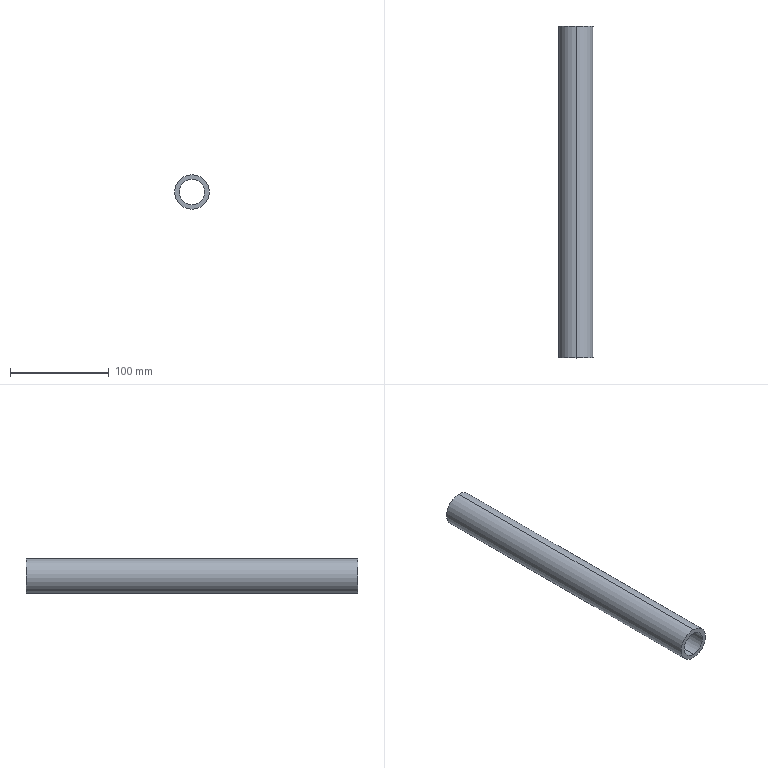Part | SolidWorks | features Extrusion 1, Shell 1 | 1 solid | 6 faces | box 35 x 337 x 35 mm | volume 145309 mm3 | cylinder 4 | plane 2 | commonest cylinder face diameters 26 x2 35 x2
STEP:
#1=CARTESIAN_POINT('',(0.,337.,-13.));
#2=VERTEX_POINT('',#1);
#3=CARTESIAN_POINT('',(0.,337.,13.));
#4=VERTEX_POINT('',#3);
#5=CARTESIAN_POINT('',(0.,337.,0.));
#6=DIRECTION('',(0.,1.,0.));
#7=DIRECTION('',(0.,0.,1.));
#8=AXIS2_PLACEMENT_3D('',#5,#6,#7);
#9=CIRCLE('',#8,13.);
#10=EDGE_CURVE('',#2,#4,#9,.T.);
#11=ORIENTED_EDGE('',*,*,#10,.T.);
#12=CARTESIAN_POINT('',(0.,0.,13.));
#13=VERTEX_POINT('',#12);
#14=CARTESIAN_POINT('',(0.,337.,13.));
#15=DIRECTION('',(0.,-1.,0.));
#16=VECTOR('',#15,1000.);
#17=LINE('',#14,#16);
#18=EDGE_CURVE('',#4,#13,#17,.T.);
#19=ORIENTED_EDGE('',*,*,#18,.T.);
#20=CARTESIAN_POINT('',(0.,0.,-13.));
#21=VERTEX_POINT('',#20);
#22=CARTESIAN_POINT('',(0.,0.,0.));
#23=DIRECTION('',(0.,1.,0.));
#24=DIRECTION('',(0.,0.,1.));
#25=AXIS2_PLACEMENT_3D('',#22,#23,#24);
#26=CIRCLE('',#25,13.);
#27=EDGE_CURVE('',#21,#13,#26,.T.);
#28=ORIENTED_EDGE('',*,*,#27,.F.);
#29=CARTESIAN_POINT('',(0.,337.,-13.));
#30=DIRECTION('',(0.,-1.,0.));
#31=VECTOR('',#30,1000.);
#32=LINE('',#29,#31);
#33=EDGE_CURVE('',#2,#21,#32,.T.);
#34=ORIENTED_EDGE('',*,*,#33,.F.);
#35=EDGE_LOOP('',(#11,#19,#28,#34));
#36=FACE_OUTER_BOUND('',#35,.T.);
#37=CARTESIAN_POINT('',(0.,337.,0.));
#38=DIRECTION('',(0.,-1.,0.));
#39=DIRECTION('',(0.,0.,-1.));
#40=AXIS2_PLACEMENT_3D('',#37,#38,#39);
#41=CYLINDRICAL_SURFACE('',#40,13.);
#42=ADVANCED_FACE('',(#36),#41,.F.);
#43=CARTESIAN_POINT('',(0.,337.,17.5));
#44=VERTEX_POINT('',#43);
#45=CARTESIAN_POINT('',(0.,337.,-17.5));
#46=VERTEX_POINT('',#45);
#47=CARTESIAN_POINT('',(0.,337.,0.));
#48=DIRECTION('',(0.,1.,0.));
#49=DIRECTION('',(0.,0.,1.));
#50=AXIS2_PLACEMENT_3D('',#47,#48,#49);
#51=CIRCLE('',#50,17.5);
#52=EDGE_CURVE('',#44,#46,#51,.T.);
#53=ORIENTED_EDGE('',*,*,#52,.F.);
#54=CARTESIAN_POINT('',(0.,0.,17.5));
#55=VERTEX_POINT('',#54);
#56=CARTESIAN_POINT('',(0.,337.,17.5));
#57=DIRECTION('',(0.,-1.,0.));
#58=VECTOR('',#57,1000.);
#59=LINE('',#56,#58);
#60=EDGE_CURVE('',#44,#55,#59,.T.);
#61=ORIENTED_EDGE('',*,*,#60,.T.);
#62=CARTESIAN_POINT('',(0.,0.,-17.5));
#63=VERTEX_POINT('',#62);
#64=CARTESIAN_POINT('',(0.,0.,0.));
#65=DIRECTION('',(0.,1.,0.));
#66=DIRECTION('',(0.,0.,1.));
#67=AXIS2_PLACEMENT_3D('',#64,#65,#66);
#68=CIRCLE('',#67,17.5);
#69=EDGE_CURVE('',#55,#63,#68,.T.);
#70=ORIENTED_EDGE('',*,*,#69,.T.);
#71=CARTESIAN_POINT('',(0.,337.,-17.5));
#72=DIRECTION('',(0.,-1.,0.));
#73=VECTOR('',#72,1000.);
#74=LINE('',#71,#73);
#75=EDGE_CURVE('',#46,#63,#74,.T.);
#76=ORIENTED_EDGE('',*,*,#75,.F.);
#77=EDGE_LOOP('',(#53,#61,#70,#76));
#78=FACE_OUTER_BOUND('',#77,.T.);
#79=CARTESIAN_POINT('',(0.,337.,0.));
#80=DIRECTION('',(0.,-1.,0.));
#81=DIRECTION('',(0.,0.,-1.));
#82=AXIS2_PLACEMENT_3D('',#79,#80,#81);
#83=CYLINDRICAL_SURFACE('',#82,17.5);
#84=ADVANCED_FACE('',(#78),#83,.T.);
#85=ORIENTED_EDGE('',*,*,#60,.F.);
#86=CARTESIAN_POINT('',(0.,337.,0.));
#87=DIRECTION('',(0.,1.,0.));
#88=DIRECTION('',(0.,0.,1.));
#89=AXIS2_PLACEMENT_3D('',#86,#87,#88);
#90=CIRCLE('',#89,17.5);
#91=EDGE_CURVE('',#46,#44,#90,.T.);
#92=ORIENTED_EDGE('',*,*,#91,.F.);
#93=ORIENTED_EDGE('',*,*,#75,.T.);
#94=CARTESIAN_POINT('',(0.,0.,0.));
#95=DIRECTION('',(0.,1.,0.));
#96=DIRECTION('',(0.,0.,1.));
#97=AXIS2_PLACEMENT_3D('',#94,#95,#96);
#98=CIRCLE('',#97,17.5);
#99=EDGE_CURVE('',#63,#55,#98,.T.);
#100=ORIENTED_EDGE('',*,*,#99,.T.);
#101=EDGE_LOOP('',(#85,#92,#93,#100));
#102=FACE_OUTER_BOUND('',#101,.T.);
#103=CARTESIAN_POINT('',(0.,337.,0.));
#104=DIRECTION('',(0.,-1.,0.));
#105=DIRECTION('',(0.,0.,-1.));
#106=AXIS2_PLACEMENT_3D('',#103,#104,#105);
#107=CYLINDRICAL_SURFACE('',#106,17.5);
#108=ADVANCED_FACE('',(#102),#107,.T.);
#109=ORIENTED_EDGE('',*,*,#10,.F.);
#110=CARTESIAN_POINT('',(0.,337.,0.));
#111=DIRECTION('',(0.,1.,0.));
#112=DIRECTION('',(0.,0.,1.));
#113=AXIS2_PLACEMENT_3D('',#110,#111,#112);
#114=CIRCLE('',#113,13.);
#115=EDGE_CURVE('',#4,#2,#114,.T.);
#116=ORIENTED_EDGE('',*,*,#115,.F.);
#117=EDGE_LOOP('',(#109,#116));
#118=FACE_BOUND('',#117,.T.);
#119=ORIENTED_EDGE('',*,*,#91,.T.);
#120=ORIENTED_EDGE('',*,*,#52,.T.);
#121=EDGE_LOOP('',(#119,#120));
#122=FACE_OUTER_BOUND('',#121,.T.);
#123=CARTESIAN_POINT('',(0.,337.,0.));
#124=DIRECTION('',(0.,1.,0.));
#125=DIRECTION('',(0.,0.,1.));
#126=AXIS2_PLACEMENT_3D('',#123,#124,#125);
#127=PLANE('',#126);
#128=ADVANCED_FACE('',(#118,#122),#127,.T.);
#129=ORIENTED_EDGE('',*,*,#27,.T.);
#130=CARTESIAN_POINT('',(0.,0.,0.));
#131=DIRECTION('',(0.,1.,0.));
#132=DIRECTION('',(0.,0.,1.));
#133=AXIS2_PLACEMENT_3D('',#130,#131,#132);
#134=CIRCLE('',#133,13.);
#135=EDGE_CURVE('',#13,#21,#134,.T.);
#136=ORIENTED_EDGE('',*,*,#135,.T.);
#137=EDGE_LOOP('',(#129,#136));
#138=FACE_BOUND('',#137,.T.);
#139=ORIENTED_EDGE('',*,*,#99,.F.);
#140=ORIENTED_EDGE('',*,*,#69,.F.);
#141=EDGE_LOOP('',(#139,#140));
#142=FACE_OUTER_BOUND('',#141,.T.);
#143=CARTESIAN_POINT('',(0.,0.,0.));
#144=DIRECTION('',(0.,1.,0.));
#145=DIRECTION('',(0.,0.,1.));
#146=AXIS2_PLACEMENT_3D('',#143,#144,#145);
#147=PLANE('',#146);
#148=ADVANCED_FACE('',(#138,#142),#147,.F.);
#149=ORIENTED_EDGE('',*,*,#18,.F.);
#150=ORIENTED_EDGE('',*,*,#115,.T.);
#151=ORIENTED_EDGE('',*,*,#33,.T.);
#152=ORIENTED_EDGE('',*,*,#135,.F.);
#153=EDGE_LOOP('',(#149,#150,#151,#152));
#154=FACE_OUTER_BOUND('',#153,.T.);
#155=CARTESIAN_POINT('',(0.,337.,0.));
#156=DIRECTION('',(0.,-1.,0.));
#157=DIRECTION('',(0.,0.,-1.));
#158=AXIS2_PLACEMENT_3D('',#155,#156,#157);
#159=CYLINDRICAL_SURFACE('',#158,13.);
#160=ADVANCED_FACE('',(#154),#159,.F.);
#161=CLOSED_SHELL('',(#42,#84,#108,#128,#148,#160));
#162=MANIFOLD_SOLID_BREP('',#161);
#163=CARTESIAN_POINT('',(0.,0.,0.));
#164=DIRECTION('',(0.,0.,1.));
#165=DIRECTION('',(1.,0.,0.));
#166=AXIS2_PLACEMENT_3D('',#163,#164,#165);
#167=(LENGTH_UNIT()NAMED_UNIT(*)SI_UNIT(.MILLI.,.METRE.));
#168=UNCERTAINTY_MEASURE_WITH_UNIT(LENGTH_MEASURE(0.00001),#167,'','');
#169=(NAMED_UNIT(*)PLANE_ANGLE_UNIT()SI_UNIT($,.RADIAN.));
#170=(NAMED_UNIT(*)SI_UNIT($,.STERADIAN.)SOLID_ANGLE_UNIT());
#171=(GEOMETRIC_REPRESENTATION_CONTEXT(3)GLOBAL_UNCERTAINTY_ASSIGNED_CONTEXT((#168))GLOBAL_UNIT_ASSIGNED_CONTEXT((#167,#169,#170))REPRESENTATION_CONTEXT('',''));
#172=ADVANCED_BREP_SHAPE_REPRESENTATION('',(#162,#166),#171);